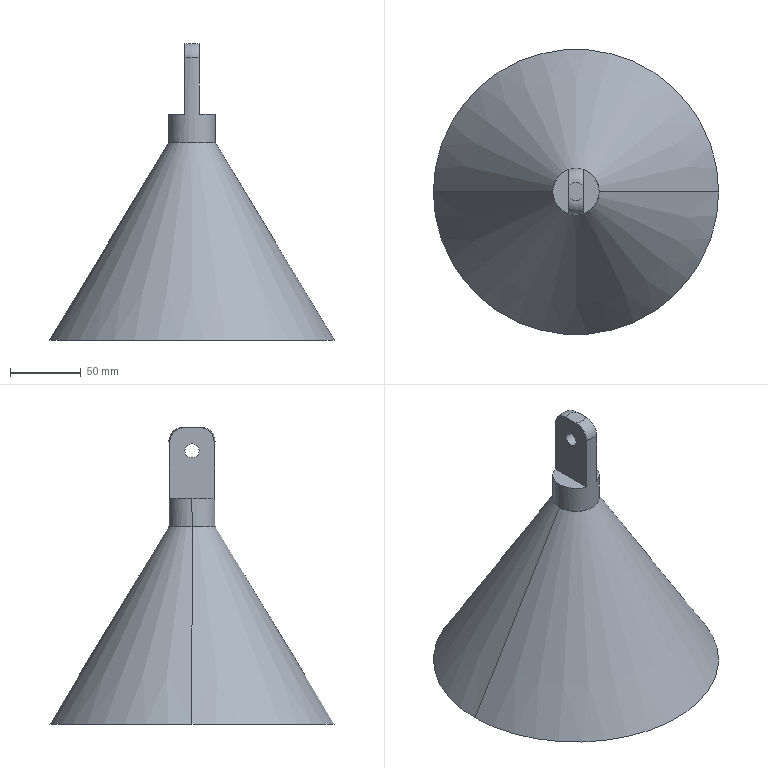Part | SolidWorks | features ICE 2, Fillet 1, RevCut 1, Revolution 1 | 1 solid | 17 faces | box 201.428 x 201.428 x 209.626 mm | volume 565522 mm3 | plane 7 | cone 4 | cylinder 4 | torus 2 | commonest cylinder face diameters 10 x2 32.806 x2
STEP:
#1=CARTESIAN_POINT('',(14.067,0.,-77.001));
#2=VERTEX_POINT('',#1);
#3=CARTESIAN_POINT('',(-14.067,0.,-77.001));
#4=VERTEX_POINT('',#3);
#5=CARTESIAN_POINT('',(0.,0.,-77.001));
#6=DIRECTION('',(0.,0.,-1.));
#7=DIRECTION('',(-1.,0.,0.));
#8=AXIS2_PLACEMENT_3D('',#5,#6,#7);
#9=CIRCLE('',#8,14.067);
#10=EDGE_CURVE('',#2,#4,#9,.T.);
#11=ORIENTED_EDGE('',*,*,#10,.F.);
#12=CARTESIAN_POINT('',(86.352,0.,-209.626));
#13=VERTEX_POINT('',#12);
#14=CARTESIAN_POINT('',(99.182,0.,-233.165));
#15=DIRECTION('',(0.4786,0.,-0.8781));
#16=VECTOR('',#15,1000.);
#17=LINE('',#14,#16);
#18=EDGE_CURVE('',#2,#13,#17,.T.);
#19=ORIENTED_EDGE('',*,*,#18,.T.);
#20=CARTESIAN_POINT('',(-86.352,0.,-209.626));
#21=VERTEX_POINT('',#20);
#22=CARTESIAN_POINT('',(0.,0.,-209.626));
#23=DIRECTION('',(0.,0.,-1.));
#24=DIRECTION('',(-1.,0.,0.));
#25=AXIS2_PLACEMENT_3D('',#22,#23,#24);
#26=CIRCLE('',#25,86.352);
#27=EDGE_CURVE('',#13,#21,#26,.T.);
#28=ORIENTED_EDGE('',*,*,#27,.T.);
#29=CARTESIAN_POINT('',(-99.182,0.,-233.165));
#30=DIRECTION('',(-0.4786,0.,-0.8781));
#31=VECTOR('',#30,1000.);
#32=LINE('',#29,#31);
#33=EDGE_CURVE('',#4,#21,#32,.T.);
#34=ORIENTED_EDGE('',*,*,#33,.F.);
#35=EDGE_LOOP('',(#11,#19,#28,#34));
#36=FACE_OUTER_BOUND('',#35,.T.);
#37=CARTESIAN_POINT('',(0.,0.,-233.165));
#38=DIRECTION('',(0.,0.,-1.));
#39=DIRECTION('',(-1.,0.,0.));
#40=AXIS2_PLACEMENT_3D('',#37,#38,#39);
#41=CONICAL_SURFACE('',#40,99.182,0.499);
#42=ADVANCED_FACE('',(#36),#41,.F.);
#43=CARTESIAN_POINT('',(-5.,-5.,-16.498));
#44=VERTEX_POINT('',#43);
#45=CARTESIAN_POINT('',(-5.,5.,-16.498));
#46=VERTEX_POINT('',#45);
#47=CARTESIAN_POINT('',(-5.,0.,-16.498));
#48=DIRECTION('',(1.,0.,0.));
#49=DIRECTION('',(0.,1.,0.));
#50=AXIS2_PLACEMENT_3D('',#47,#48,#49);
#51=CIRCLE('',#50,5.);
#52=EDGE_CURVE('',#44,#46,#51,.T.);
#53=ORIENTED_EDGE('',*,*,#52,.F.);
#54=CARTESIAN_POINT('',(5.,-5.,-16.498));
#55=VERTEX_POINT('',#54);
#56=CARTESIAN_POINT('',(-45.,-5.,-16.498));
#57=DIRECTION('',(1.,0.,0.));
#58=VECTOR('',#57,1000.);
#59=LINE('',#56,#58);
#60=EDGE_CURVE('',#44,#55,#59,.T.);
#61=ORIENTED_EDGE('',*,*,#60,.T.);
#62=CARTESIAN_POINT('',(5.,5.,-16.498));
#63=VERTEX_POINT('',#62);
#64=CARTESIAN_POINT('',(5.,0.,-16.498));
#65=DIRECTION('',(1.,0.,0.));
#66=DIRECTION('',(0.,1.,0.));
#67=AXIS2_PLACEMENT_3D('',#64,#65,#66);
#68=CIRCLE('',#67,5.);
#69=EDGE_CURVE('',#55,#63,#68,.T.);
#70=ORIENTED_EDGE('',*,*,#69,.T.);
#71=CARTESIAN_POINT('',(-45.,5.,-16.498));
#72=DIRECTION('',(1.,0.,0.));
#73=VECTOR('',#72,1000.);
#74=LINE('',#71,#73);
#75=EDGE_CURVE('',#46,#63,#74,.T.);
#76=ORIENTED_EDGE('',*,*,#75,.F.);
#77=EDGE_LOOP('',(#53,#61,#70,#76));
#78=FACE_OUTER_BOUND('',#77,.T.);
#79=CARTESIAN_POINT('',(-45.,0.,-16.498));
#80=DIRECTION('',(1.,0.,0.));
#81=DIRECTION('',(0.,1.,0.));
#82=AXIS2_PLACEMENT_3D('',#79,#80,#81);
#83=CYLINDRICAL_SURFACE('',#82,5.);
#84=ADVANCED_FACE('',(#78),#83,.F.);
#85=CARTESIAN_POINT('',(16.403,0.,-69.874));
#86=VERTEX_POINT('',#85);
#87=CARTESIAN_POINT('',(-16.403,0.,-69.874));
#88=VERTEX_POINT('',#87);
#89=CARTESIAN_POINT('',(0.,0.,-69.874));
#90=DIRECTION('',(0.,0.,1.));
#91=DIRECTION('',(1.,0.,0.));
#92=AXIS2_PLACEMENT_3D('',#89,#90,#91);
#93=CIRCLE('',#92,16.403);
#94=EDGE_CURVE('',#86,#88,#93,.T.);
#95=ORIENTED_EDGE('',*,*,#94,.T.);
#96=CARTESIAN_POINT('',(-16.403,0.,-50.));
#97=VERTEX_POINT('',#96);
#98=CARTESIAN_POINT('',(-16.403,0.,0.));
#99=DIRECTION('',(0.,0.,1.));
#100=VECTOR('',#99,1000.);
#101=LINE('',#98,#100);
#102=EDGE_CURVE('',#88,#97,#101,.T.);
#103=ORIENTED_EDGE('',*,*,#102,.T.);
#104=CARTESIAN_POINT('',(-5.,15.622,-50.));
#105=VERTEX_POINT('',#104);
#106=CARTESIAN_POINT('',(0.,0.,-50.));
#107=DIRECTION('',(0.,0.,-1.));
#108=DIRECTION('',(1.,0.,0.));
#109=AXIS2_PLACEMENT_3D('',#106,#107,#108);
#110=CIRCLE('',#109,16.403);
#111=EDGE_CURVE('',#97,#105,#110,.T.);
#112=ORIENTED_EDGE('',*,*,#111,.T.);
#113=CARTESIAN_POINT('',(-5.,15.622,-10.));
#114=VERTEX_POINT('',#113);
#115=CARTESIAN_POINT('',(-5.,15.622,0.));
#116=DIRECTION('',(0.,0.,-1.));
#117=VECTOR('',#116,1000.);
#118=LINE('',#115,#117);
#119=EDGE_CURVE('',#114,#105,#118,.T.);
#120=ORIENTED_EDGE('',*,*,#119,.F.);
#121=CARTESIAN_POINT('',(5.,15.622,-10.));
#122=VERTEX_POINT('',#121);
#123=CARTESIAN_POINT('',(0.,0.,-10.));
#124=DIRECTION('',(0.,0.,-1.));
#125=DIRECTION('',(1.,0.,0.));
#126=AXIS2_PLACEMENT_3D('',#123,#124,#125);
#127=CIRCLE('',#126,16.403);
#128=EDGE_CURVE('',#114,#122,#127,.T.);
#129=ORIENTED_EDGE('',*,*,#128,.T.);
#130=CARTESIAN_POINT('',(5.,15.622,-50.));
#131=VERTEX_POINT('',#130);
#132=CARTESIAN_POINT('',(5.,15.622,0.));
#133=DIRECTION('',(0.,0.,1.));
#134=VECTOR('',#133,1000.);
#135=LINE('',#132,#134);
#136=EDGE_CURVE('',#131,#122,#135,.T.);
#137=ORIENTED_EDGE('',*,*,#136,.F.);
#138=CARTESIAN_POINT('',(16.403,0.,-50.));
#139=VERTEX_POINT('',#138);
#140=CARTESIAN_POINT('',(0.,0.,-50.));
#141=DIRECTION('',(0.,0.,-1.));
#142=DIRECTION('',(1.,0.,0.));
#143=AXIS2_PLACEMENT_3D('',#140,#141,#142);
#144=CIRCLE('',#143,16.403);
#145=EDGE_CURVE('',#131,#139,#144,.T.);
#146=ORIENTED_EDGE('',*,*,#145,.T.);
#147=CARTESIAN_POINT('',(16.403,0.,0.));
#148=DIRECTION('',(0.,0.,1.));
#149=VECTOR('',#148,1000.);
#150=LINE('',#147,#149);
#151=EDGE_CURVE('',#86,#139,#150,.T.);
#152=ORIENTED_EDGE('',*,*,#151,.F.);
#153=EDGE_LOOP('',(#95,#103,#112,#120,#129,#137,#146,#152));
#154=FACE_OUTER_BOUND('',#153,.T.);
#155=CARTESIAN_POINT('',(0.,0.,0.));
#156=DIRECTION('',(0.,0.,1.));
#157=DIRECTION('',(1.,0.,0.));
#158=AXIS2_PLACEMENT_3D('',#155,#156,#157);
#159=CYLINDRICAL_SURFACE('',#158,16.403);
#160=ADVANCED_FACE('',(#154),#159,.T.);
#161=ORIENTED_EDGE('',*,*,#94,.F.);
#162=CARTESIAN_POINT('',(100.714,0.,-209.626));
#163=VERTEX_POINT('',#162);
#164=CARTESIAN_POINT('',(16.403,0.,-69.874));
#165=DIRECTION('',(0.5166,0.,-0.8562));
#166=VECTOR('',#165,1000.);
#167=LINE('',#164,#166);
#168=EDGE_CURVE('',#86,#163,#167,.T.);
#169=ORIENTED_EDGE('',*,*,#168,.T.);
#170=CARTESIAN_POINT('',(-100.714,0.,-209.626));
#171=VERTEX_POINT('',#170);
#172=CARTESIAN_POINT('',(0.,0.,-209.626));
#173=DIRECTION('',(0.,0.,1.));
#174=DIRECTION('',(1.,0.,0.));
#175=AXIS2_PLACEMENT_3D('',#172,#173,#174);
#176=CIRCLE('',#175,100.714);
#177=EDGE_CURVE('',#163,#171,#176,.T.);
#178=ORIENTED_EDGE('',*,*,#177,.T.);
#179=CARTESIAN_POINT('',(-16.403,0.,-69.874));
#180=DIRECTION('',(-0.5166,0.,-0.8562));
#181=VECTOR('',#180,1000.);
#182=LINE('',#179,#181);
#183=EDGE_CURVE('',#88,#171,#182,.T.);
#184=ORIENTED_EDGE('',*,*,#183,.F.);
#185=EDGE_LOOP('',(#161,#169,#178,#184));
#186=FACE_OUTER_BOUND('',#185,.T.);
#187=CARTESIAN_POINT('',(0.,0.,-69.874));
#188=DIRECTION('',(0.,0.,-1.));
#189=DIRECTION('',(-1.,0.,0.));
#190=AXIS2_PLACEMENT_3D('',#187,#188,#189);
#191=CONICAL_SURFACE('',#190,16.403,0.5428);
#192=ADVANCED_FACE('',(#186),#191,.T.);
#193=CARTESIAN_POINT('',(0.,0.,-209.626));
#194=DIRECTION('',(0.,0.,-1.));
#195=DIRECTION('',(-1.,0.,0.));
#196=AXIS2_PLACEMENT_3D('',#193,#194,#195);
#197=CIRCLE('',#196,86.352);
#198=EDGE_CURVE('',#21,#13,#197,.T.);
#199=ORIENTED_EDGE('',*,*,#198,.F.);
#200=ORIENTED_EDGE('',*,*,#27,.F.);
#201=EDGE_LOOP('',(#199,#200));
#202=FACE_BOUND('',#201,.T.);
#203=CARTESIAN_POINT('',(0.,0.,-209.626));
#204=DIRECTION('',(0.,0.,1.));
#205=DIRECTION('',(1.,0.,0.));
#206=AXIS2_PLACEMENT_3D('',#203,#204,#205);
#207=CIRCLE('',#206,100.714);
#208=EDGE_CURVE('',#171,#163,#207,.T.);
#209=ORIENTED_EDGE('',*,*,#208,.F.);
#210=ORIENTED_EDGE('',*,*,#177,.F.);
#211=EDGE_LOOP('',(#209,#210));
#212=FACE_OUTER_BOUND('',#211,.T.);
#213=CARTESIAN_POINT('',(100.714,0.,-209.626));
#214=DIRECTION('',(0.,0.,-1.));
#215=DIRECTION('',(-1.,0.,0.));
#216=AXIS2_PLACEMENT_3D('',#213,#214,#215);
#217=PLANE('',#216);
#218=ADVANCED_FACE('',(#202,#212),#217,.T.);
#219=ORIENTED_EDGE('',*,*,#168,.F.);
#220=CARTESIAN_POINT('',(0.,0.,-69.874));
#221=DIRECTION('',(0.,0.,1.));
#222=DIRECTION('',(1.,0.,0.));
#223=AXIS2_PLACEMENT_3D('',#220,#221,#222);
#224=CIRCLE('',#223,16.403);
#225=EDGE_CURVE('',#88,#86,#224,.T.);
#226=ORIENTED_EDGE('',*,*,#225,.F.);
#227=ORIENTED_EDGE('',*,*,#183,.T.);
#228=ORIENTED_EDGE('',*,*,#208,.T.);
#229=EDGE_LOOP('',(#219,#226,#227,#228));
#230=FACE_OUTER_BOUND('',#229,.T.);
#231=CARTESIAN_POINT('',(0.,0.,-69.874));
#232=DIRECTION('',(0.,0.,-1.));
#233=DIRECTION('',(-1.,0.,0.));
#234=AXIS2_PLACEMENT_3D('',#231,#232,#233);
#235=CONICAL_SURFACE('',#234,16.403,0.5428);
#236=ADVANCED_FACE('',(#230),#235,.T.);
#237=ORIENTED_EDGE('',*,*,#102,.F.);
#238=ORIENTED_EDGE('',*,*,#225,.T.);
#239=ORIENTED_EDGE('',*,*,#151,.T.);
#240=CARTESIAN_POINT('',(5.,-15.622,-50.));
#241=VERTEX_POINT('',#240);
#242=CARTESIAN_POINT('',(0.,0.,-50.));
#243=DIRECTION('',(0.,0.,-1.));
#244=DIRECTION('',(1.,0.,0.));
#245=AXIS2_PLACEMENT_3D('',#242,#243,#244);
#246=CIRCLE('',#245,16.403);
#247=EDGE_CURVE('',#139,#241,#246,.T.);
#248=ORIENTED_EDGE('',*,*,#247,.T.);
#249=CARTESIAN_POINT('',(5.,-15.622,-10.));
#250=VERTEX_POINT('',#249);
#251=CARTESIAN_POINT('',(5.,-15.622,0.));
#252=DIRECTION('',(0.,0.,-1.));
#253=VECTOR('',#252,1000.);
#254=LINE('',#251,#253);
#255=EDGE_CURVE('',#250,#241,#254,.T.);
#256=ORIENTED_EDGE('',*,*,#255,.F.);
#257=CARTESIAN_POINT('',(-5.,-15.622,-10.));
#258=VERTEX_POINT('',#257);
#259=CARTESIAN_POINT('',(0.,0.,-10.));
#260=DIRECTION('',(0.,0.,-1.));
#261=DIRECTION('',(1.,0.,0.));
#262=AXIS2_PLACEMENT_3D('',#259,#260,#261);
#263=CIRCLE('',#262,16.403);
#264=EDGE_CURVE('',#250,#258,#263,.T.);
#265=ORIENTED_EDGE('',*,*,#264,.T.);
#266=CARTESIAN_POINT('',(-5.,-15.622,-50.));
#267=VERTEX_POINT('',#266);
#268=CARTESIAN_POINT('',(-5.,-15.622,0.));
#269=DIRECTION('',(0.,0.,1.));
#270=VECTOR('',#269,1000.);
#271=LINE('',#268,#270);
#272=EDGE_CURVE('',#267,#258,#271,.T.);
#273=ORIENTED_EDGE('',*,*,#272,.F.);
#274=CARTESIAN_POINT('',(0.,0.,-50.));
#275=DIRECTION('',(0.,0.,-1.));
#276=DIRECTION('',(1.,0.,0.));
#277=AXIS2_PLACEMENT_3D('',#274,#275,#276);
#278=CIRCLE('',#277,16.403);
#279=EDGE_CURVE('',#267,#97,#278,.T.);
#280=ORIENTED_EDGE('',*,*,#279,.T.);
#281=EDGE_LOOP('',(#237,#238,#239,#248,#256,#265,#273,#280));
#282=FACE_OUTER_BOUND('',#281,.T.);
#283=CARTESIAN_POINT('',(0.,0.,0.));
#284=DIRECTION('',(0.,0.,1.));
#285=DIRECTION('',(1.,0.,0.));
#286=AXIS2_PLACEMENT_3D('',#283,#284,#285);
#287=CYLINDRICAL_SURFACE('',#286,16.403);
#288=ADVANCED_FACE('',(#282),#287,.T.);
#289=CARTESIAN_POINT('',(-5.,-4.,0.));
#290=VERTEX_POINT('',#289);
#291=CARTESIAN_POINT('',(-5.,4.,0.));
#292=VERTEX_POINT('',#291);
#293=CARTESIAN_POINT('',(-5.,0.,0.));
#294=DIRECTION('',(0.,1.,0.));
#295=VECTOR('',#294,1000.);
#296=LINE('',#293,#295);
#297=EDGE_CURVE('',#290,#292,#296,.T.);
#298=ORIENTED_EDGE('',*,*,#297,.F.);
#299=CARTESIAN_POINT('',(5.,-4.,0.));
#300=VERTEX_POINT('',#299);
#301=CARTESIAN_POINT('',(0.,0.,0.));
#302=DIRECTION('',(0.,0.,1.));
#303=DIRECTION('',(1.,0.,0.));
#304=AXIS2_PLACEMENT_3D('',#301,#302,#303);
#305=CIRCLE('',#304,6.403);
#306=EDGE_CURVE('',#290,#300,#305,.T.);
#307=ORIENTED_EDGE('',*,*,#306,.T.);
#308=CARTESIAN_POINT('',(5.,4.,0.));
#309=VERTEX_POINT('',#308);
#310=CARTESIAN_POINT('',(5.,0.,0.));
#311=DIRECTION('',(0.,-1.,0.));
#312=VECTOR('',#311,1000.);
#313=LINE('',#310,#312);
#314=EDGE_CURVE('',#309,#300,#313,.T.);
#315=ORIENTED_EDGE('',*,*,#314,.F.);
#316=CARTESIAN_POINT('',(0.,0.,0.));
#317=DIRECTION('',(0.,0.,1.));
#318=DIRECTION('',(1.,0.,0.));
#319=AXIS2_PLACEMENT_3D('',#316,#317,#318);
#320=CIRCLE('',#319,6.403);
#321=EDGE_CURVE('',#309,#292,#320,.T.);
#322=ORIENTED_EDGE('',*,*,#321,.T.);
#323=EDGE_LOOP('',(#298,#307,#315,#322));
#324=FACE_OUTER_BOUND('',#323,.T.);
#325=CARTESIAN_POINT('',(0.,0.,0.));
#326=DIRECTION('',(0.,0.,1.));
#327=DIRECTION('',(1.,0.,0.));
#328=AXIS2_PLACEMENT_3D('',#325,#326,#327);
#329=PLANE('',#328);
#330=ADVANCED_FACE('',(#324),#329,.T.);
#331=CARTESIAN_POINT('',(5.,0.,-16.498));
#332=DIRECTION('',(1.,0.,0.));
#333=DIRECTION('',(0.,1.,0.));
#334=AXIS2_PLACEMENT_3D('',#331,#332,#333);
#335=CIRCLE('',#334,5.);
#336=EDGE_CURVE('',#63,#55,#335,.T.);
#337=ORIENTED_EDGE('',*,*,#336,.F.);
#338=ORIENTED_EDGE('',*,*,#69,.F.);
#339=EDGE_LOOP('',(#337,#338));
#340=FACE_BOUND('',#339,.T.);
#341=ORIENTED_EDGE('',*,*,#314,.T.);
#342=CARTESIAN_POINT('',(5.,-4.,0.));
#343=CARTESIAN_POINT('',(5.,-4.717,0.));
#344=CARTESIAN_POINT('',(5.,-5.428,-0.03133));
#345=CARTESIAN_POINT('',(5.,-6.833,-0.1975));
#346=CARTESIAN_POINT('',(5.,-7.527,-0.3314));
#347=CARTESIAN_POINT('',(5.,-8.55,-0.6277));
#348=CARTESIAN_POINT('',(5.,-8.889,-0.7422));
#349=CARTESIAN_POINT('',(5.,-9.56,-1.006));
#350=CARTESIAN_POINT('',(5.,-9.889,-1.155));
#351=CARTESIAN_POINT('',(5.,-10.845,-1.646));
#352=CARTESIAN_POINT('',(5.,-11.445,-2.035));
#353=CARTESIAN_POINT('',(5.,-12.283,-2.715));
#354=CARTESIAN_POINT('',(5.,-12.553,-2.959));
#355=CARTESIAN_POINT('',(5.,-13.058,-3.468));
#356=CARTESIAN_POINT('',(5.,-13.296,-3.735));
#357=CARTESIAN_POINT('',(5.,-13.74,-4.293));
#358=CARTESIAN_POINT('',(5.,-13.947,-4.584));
#359=CARTESIAN_POINT('',(5.,-14.33,-5.19));
#360=CARTESIAN_POINT('',(5.,-14.507,-5.508));
#361=CARTESIAN_POINT('',(5.,-14.978,-6.48));
#362=CARTESIAN_POINT('',(5.,-15.215,-7.153));
#363=CARTESIAN_POINT('',(5.,-15.458,-8.201));
#364=CARTESIAN_POINT('',(5.,-15.519,-8.558));
#365=CARTESIAN_POINT('',(5.,-15.602,-9.277));
#366=CARTESIAN_POINT('',(5.,-15.622,-9.638));
#367=CARTESIAN_POINT('',(5.,-15.622,-10.));
#368=B_SPLINE_CURVE_WITH_KNOTS('',3,(#342,#343,#344,#345,#346,#347,#348,#349,#350,#351,#352,#353,#354,#355,#356,#357,#358,#359,#360,#361,#362,#363,#364,#365,#366,#367),.UNSPECIFIED.,.F.,.F.,(4,2,2,2,2,2,2,2,2,2,2,2,4),(0.,0.002119,0.004238,0.005297,0.006357,0.008475,0.009535,0.01059,0.01165,0.01271,0.01483,0.01589,0.01695),.UNSPECIFIED.);
#369=EDGE_CURVE('',#300,#250,#368,.T.);
#370=ORIENTED_EDGE('',*,*,#369,.T.);
#371=ORIENTED_EDGE('',*,*,#255,.T.);
#372=CARTESIAN_POINT('',(5.,19.006,-50.));
#373=DIRECTION('',(0.,-1.,0.));
#374=VECTOR('',#373,1000.);
#375=LINE('',#372,#374);
#376=EDGE_CURVE('',#131,#241,#375,.T.);
#377=ORIENTED_EDGE('',*,*,#376,.F.);
#378=ORIENTED_EDGE('',*,*,#136,.T.);
#379=CARTESIAN_POINT('',(5.,15.622,-10.));
#380=CARTESIAN_POINT('',(5.,15.622,-9.277));
#381=CARTESIAN_POINT('',(5.,15.541,-8.569));
#382=CARTESIAN_POINT('',(5.,15.223,-7.178));
#383=CARTESIAN_POINT('',(5.,14.981,-6.49));
#384=CARTESIAN_POINT('',(5.,14.361,-5.205));
#385=CARTESIAN_POINT('',(5.,13.983,-4.6));
#386=CARTESIAN_POINT('',(5.,13.086,-3.468));
#387=CARTESIAN_POINT('',(5.,12.583,-2.961));
#388=CARTESIAN_POINT('',(5.,11.478,-2.058));
#389=CARTESIAN_POINT('',(5.,10.868,-1.66));
#390=CARTESIAN_POINT('',(5.,9.599,-1.004));
#391=CARTESIAN_POINT('',(5.,8.935,-0.7415));
#392=CARTESIAN_POINT('',(5.,7.9,-0.4383));
#393=CARTESIAN_POINT('',(5.,7.549,-0.3529));
#394=CARTESIAN_POINT('',(5.,6.848,-0.2129));
#395=CARTESIAN_POINT('',(5.,6.495,-0.1577));
#396=CARTESIAN_POINT('',(5.,5.432,-0.03135));
#397=CARTESIAN_POINT('',(5.,4.718,0.));
#398=CARTESIAN_POINT('',(5.,4.,0.));
#399=B_SPLINE_CURVE_WITH_KNOTS('',3,(#379,#380,#381,#382,#383,#384,#385,#386,#387,#388,#389,#390,#391,#392,#393,#394,#395,#396,#397,#398),.UNSPECIFIED.,.F.,.F.,(4,2,2,2,2,2,2,2,2,4),(0.,0.002137,0.004273,0.00641,0.008547,0.01068,0.01282,0.01389,0.01496,0.01709),.UNSPECIFIED.);
#400=EDGE_CURVE('',#122,#309,#399,.T.);
#401=ORIENTED_EDGE('',*,*,#400,.T.);
#402=EDGE_LOOP('',(#341,#370,#371,#377,#378,#401));
#403=FACE_OUTER_BOUND('',#402,.T.);
#404=CARTESIAN_POINT('',(5.,19.006,-50.));
#405=DIRECTION('',(-1.,0.,0.));
#406=DIRECTION('',(0.,-1.,0.));
#407=AXIS2_PLACEMENT_3D('',#404,#405,#406);
#408=PLANE('',#407);
#409=ADVANCED_FACE('',(#340,#403),#408,.F.);
#410=ORIENTED_EDGE('',*,*,#376,.T.);
#411=ORIENTED_EDGE('',*,*,#247,.F.);
#412=ORIENTED_EDGE('',*,*,#145,.F.);
#413=EDGE_LOOP('',(#410,#411,#412));
#414=FACE_OUTER_BOUND('',#413,.T.);
#415=CARTESIAN_POINT('',(0.,0.,-50.));
#416=DIRECTION('',(0.,0.,1.));
#417=DIRECTION('',(1.,0.,0.));
#418=AXIS2_PLACEMENT_3D('',#415,#416,#417);
#419=PLANE('',#418);
#420=ADVANCED_FACE('',(#414),#419,.T.);
#421=CARTESIAN_POINT('',(-5.,0.,-16.498));
#422=DIRECTION('',(1.,0.,0.));
#423=DIRECTION('',(0.,1.,0.));
#424=AXIS2_PLACEMENT_3D('',#421,#422,#423);
#425=CIRCLE('',#424,5.);
#426=EDGE_CURVE('',#46,#44,#425,.T.);
#427=ORIENTED_EDGE('',*,*,#426,.T.);
#428=ORIENTED_EDGE('',*,*,#52,.T.);
#429=EDGE_LOOP('',(#427,#428));
#430=FACE_BOUND('',#429,.T.);
#431=ORIENTED_EDGE('',*,*,#272,.T.);
#432=CARTESIAN_POINT('',(-5.,-15.622,-10.));
#433=CARTESIAN_POINT('',(-5.,-15.622,-9.277));
#434=CARTESIAN_POINT('',(-5.,-15.541,-8.569));
#435=CARTESIAN_POINT('',(-5.,-15.223,-7.178));
#436=CARTESIAN_POINT('',(-5.,-14.981,-6.49));
#437=CARTESIAN_POINT('',(-5.,-14.361,-5.205));
#438=CARTESIAN_POINT('',(-5.,-13.983,-4.6));
#439=CARTESIAN_POINT('',(-5.,-13.086,-3.468));
#440=CARTESIAN_POINT('',(-5.,-12.583,-2.961));
#441=CARTESIAN_POINT('',(-5.,-11.478,-2.058));
#442=CARTESIAN_POINT('',(-5.,-10.868,-1.66));
#443=CARTESIAN_POINT('',(-5.,-9.599,-1.004));
#444=CARTESIAN_POINT('',(-5.,-8.935,-0.7415));
#445=CARTESIAN_POINT('',(-5.,-7.9,-0.4383));
#446=CARTESIAN_POINT('',(-5.,-7.549,-0.3529));
#447=CARTESIAN_POINT('',(-5.,-6.848,-0.2129));
#448=CARTESIAN_POINT('',(-5.,-6.495,-0.1577));
#449=CARTESIAN_POINT('',(-5.,-5.432,-0.03135));
#450=CARTESIAN_POINT('',(-5.,-4.718,0.));
#451=CARTESIAN_POINT('',(-5.,-4.,0.));
#452=B_SPLINE_CURVE_WITH_KNOTS('',3,(#432,#433,#434,#435,#436,#437,#438,#439,#440,#441,#442,#443,#444,#445,#446,#447,#448,#449,#450,#451),.UNSPECIFIED.,.F.,.F.,(4,2,2,2,2,2,2,2,2,4),(0.,0.002137,0.004273,0.00641,0.008547,0.01068,0.01282,0.01389,0.01496,0.01709),.UNSPECIFIED.);
#453=EDGE_CURVE('',#258,#290,#452,.T.);
#454=ORIENTED_EDGE('',*,*,#453,.T.);
#455=ORIENTED_EDGE('',*,*,#297,.T.);
#456=CARTESIAN_POINT('',(-5.,4.,0.));
#457=CARTESIAN_POINT('',(-5.,4.717,0.));
#458=CARTESIAN_POINT('',(-5.,5.428,-0.03133));
#459=CARTESIAN_POINT('',(-5.,6.833,-0.1975));
#460=CARTESIAN_POINT('',(-5.,7.527,-0.3314));
#461=CARTESIAN_POINT('',(-5.,8.55,-0.6277));
#462=CARTESIAN_POINT('',(-5.,8.889,-0.7422));
#463=CARTESIAN_POINT('',(-5.,9.56,-1.006));
#464=CARTESIAN_POINT('',(-5.,9.889,-1.155));
#465=CARTESIAN_POINT('',(-5.,10.845,-1.646));
#466=CARTESIAN_POINT('',(-5.,11.445,-2.035));
#467=CARTESIAN_POINT('',(-5.,12.283,-2.715));
#468=CARTESIAN_POINT('',(-5.,12.553,-2.959));
#469=CARTESIAN_POINT('',(-5.,13.058,-3.468));
#470=CARTESIAN_POINT('',(-5.,13.296,-3.735));
#471=CARTESIAN_POINT('',(-5.,13.74,-4.293));
#472=CARTESIAN_POINT('',(-5.,13.947,-4.584));
#473=CARTESIAN_POINT('',(-5.,14.33,-5.19));
#474=CARTESIAN_POINT('',(-5.,14.507,-5.508));
#475=CARTESIAN_POINT('',(-5.,14.978,-6.48));
#476=CARTESIAN_POINT('',(-5.,15.215,-7.153));
#477=CARTESIAN_POINT('',(-5.,15.458,-8.201));
#478=CARTESIAN_POINT('',(-5.,15.519,-8.558));
#479=CARTESIAN_POINT('',(-5.,15.602,-9.277));
#480=CARTESIAN_POINT('',(-5.,15.622,-9.638));
#481=CARTESIAN_POINT('',(-5.,15.622,-10.));
#482=B_SPLINE_CURVE_WITH_KNOTS('',3,(#456,#457,#458,#459,#460,#461,#462,#463,#464,#465,#466,#467,#468,#469,#470,#471,#472,#473,#474,#475,#476,#477,#478,#479,#480,#481),.UNSPECIFIED.,.F.,.F.,(4,2,2,2,2,2,2,2,2,2,2,2,4),(0.,0.002119,0.004238,0.005297,0.006357,0.008475,0.009535,0.01059,0.01165,0.01271,0.01483,0.01589,0.01695),.UNSPECIFIED.);
#483=EDGE_CURVE('',#292,#114,#482,.T.);
#484=ORIENTED_EDGE('',*,*,#483,.T.);
#485=ORIENTED_EDGE('',*,*,#119,.T.);
#486=CARTESIAN_POINT('',(-5.,19.006,-50.));
#487=DIRECTION('',(0.,1.,0.));
#488=VECTOR('',#487,1000.);
#489=LINE('',#486,#488);
#490=EDGE_CURVE('',#267,#105,#489,.T.);
#491=ORIENTED_EDGE('',*,*,#490,.F.);
#492=EDGE_LOOP('',(#431,#454,#455,#484,#485,#491));
#493=FACE_OUTER_BOUND('',#492,.T.);
#494=CARTESIAN_POINT('',(-5.,19.006,-50.));
#495=DIRECTION('',(1.,0.,0.));
#496=DIRECTION('',(0.,1.,0.));
#497=AXIS2_PLACEMENT_3D('',#494,#495,#496);
#498=PLANE('',#497);
#499=ADVANCED_FACE('',(#430,#493),#498,.F.);
#500=ORIENTED_EDGE('',*,*,#490,.T.);
#501=ORIENTED_EDGE('',*,*,#111,.F.);
#502=ORIENTED_EDGE('',*,*,#279,.F.);
#503=EDGE_LOOP('',(#500,#501,#502));
#504=FACE_OUTER_BOUND('',#503,.T.);
#505=CARTESIAN_POINT('',(0.,0.,-50.));
#506=DIRECTION('',(0.,0.,1.));
#507=DIRECTION('',(1.,0.,0.));
#508=AXIS2_PLACEMENT_3D('',#505,#506,#507);
#509=PLANE('',#508);
#510=ADVANCED_FACE('',(#504),#509,.T.);
#511=ORIENTED_EDGE('',*,*,#60,.F.);
#512=ORIENTED_EDGE('',*,*,#426,.F.);
#513=ORIENTED_EDGE('',*,*,#75,.T.);
#514=ORIENTED_EDGE('',*,*,#336,.T.);
#515=EDGE_LOOP('',(#511,#512,#513,#514));
#516=FACE_OUTER_BOUND('',#515,.T.);
#517=CARTESIAN_POINT('',(-45.,0.,-16.498));
#518=DIRECTION('',(1.,0.,0.));
#519=DIRECTION('',(0.,1.,0.));
#520=AXIS2_PLACEMENT_3D('',#517,#518,#519);
#521=CYLINDRICAL_SURFACE('',#520,5.);
#522=ADVANCED_FACE('',(#516),#521,.F.);
#523=ORIENTED_EDGE('',*,*,#453,.F.);
#524=ORIENTED_EDGE('',*,*,#264,.F.);
#525=ORIENTED_EDGE('',*,*,#369,.F.);
#526=ORIENTED_EDGE('',*,*,#306,.F.);
#527=EDGE_LOOP('',(#523,#524,#525,#526));
#528=FACE_OUTER_BOUND('',#527,.T.);
#529=CARTESIAN_POINT('',(0.,0.,-10.));
#530=DIRECTION('',(0.,0.,1.));
#531=DIRECTION('',(1.,0.,0.));
#532=AXIS2_PLACEMENT_3D('',#529,#530,#531);
#533=TOROIDAL_SURFACE('',#532,6.403,10.);
#534=ADVANCED_FACE('',(#528),#533,.T.);
#535=ORIENTED_EDGE('',*,*,#400,.F.);
#536=ORIENTED_EDGE('',*,*,#128,.F.);
#537=ORIENTED_EDGE('',*,*,#483,.F.);
#538=ORIENTED_EDGE('',*,*,#321,.F.);
#539=EDGE_LOOP('',(#535,#536,#537,#538));
#540=FACE_OUTER_BOUND('',#539,.T.);
#541=CARTESIAN_POINT('',(0.,0.,-10.));
#542=DIRECTION('',(0.,0.,1.));
#543=DIRECTION('',(1.,0.,0.));
#544=AXIS2_PLACEMENT_3D('',#541,#542,#543);
#545=TOROIDAL_SURFACE('',#544,6.403,10.);
#546=ADVANCED_FACE('',(#540),#545,.T.);
#547=CARTESIAN_POINT('',(0.,0.,-77.001));
#548=DIRECTION('',(0.,0.,-1.));
#549=DIRECTION('',(-1.,0.,0.));
#550=AXIS2_PLACEMENT_3D('',#547,#548,#549);
#551=CIRCLE('',#550,14.067);
#552=EDGE_CURVE('',#4,#2,#551,.T.);
#553=ORIENTED_EDGE('',*,*,#552,.T.);
#554=ORIENTED_EDGE('',*,*,#10,.T.);
#555=EDGE_LOOP('',(#553,#554));
#556=FACE_OUTER_BOUND('',#555,.T.);
#557=CARTESIAN_POINT('',(0.,0.,-77.001));
#558=DIRECTION('',(0.,0.,1.));
#559=DIRECTION('',(1.,0.,0.));
#560=AXIS2_PLACEMENT_3D('',#557,#558,#559);
#561=PLANE('',#560);
#562=ADVANCED_FACE('',(#556),#561,.F.);
#563=ORIENTED_EDGE('',*,*,#18,.F.);
#564=ORIENTED_EDGE('',*,*,#552,.F.);
#565=ORIENTED_EDGE('',*,*,#33,.T.);
#566=ORIENTED_EDGE('',*,*,#198,.T.);
#567=EDGE_LOOP('',(#563,#564,#565,#566));
#568=FACE_OUTER_BOUND('',#567,.T.);
#569=CARTESIAN_POINT('',(0.,0.,-233.165));
#570=DIRECTION('',(0.,0.,-1.));
#571=DIRECTION('',(-1.,0.,0.));
#572=AXIS2_PLACEMENT_3D('',#569,#570,#571);
#573=CONICAL_SURFACE('',#572,99.182,0.499);
#574=ADVANCED_FACE('',(#568),#573,.F.);
#575=CLOSED_SHELL('',(#42,#84,#160,#192,#218,#236,#288,#330,#409,#420,#499,#510,#522,#534,#546,#562,#574));
#576=MANIFOLD_SOLID_BREP('',#575);
#577=CARTESIAN_POINT('',(0.,0.,0.));
#578=DIRECTION('',(0.,0.,1.));
#579=DIRECTION('',(1.,0.,0.));
#580=AXIS2_PLACEMENT_3D('',#577,#578,#579);
#581=(LENGTH_UNIT()NAMED_UNIT(*)SI_UNIT(.MILLI.,.METRE.));
#582=UNCERTAINTY_MEASURE_WITH_UNIT(LENGTH_MEASURE(0.00001),#581,'','');
#583=(NAMED_UNIT(*)PLANE_ANGLE_UNIT()SI_UNIT($,.RADIAN.));
#584=(NAMED_UNIT(*)SI_UNIT($,.STERADIAN.)SOLID_ANGLE_UNIT());
#585=(GEOMETRIC_REPRESENTATION_CONTEXT(3)GLOBAL_UNCERTAINTY_ASSIGNED_CONTEXT((#582))GLOBAL_UNIT_ASSIGNED_CONTEXT((#581,#583,#584))REPRESENTATION_CONTEXT('',''));
#586=ADVANCED_BREP_SHAPE_REPRESENTATION('',(#576,#580),#585);